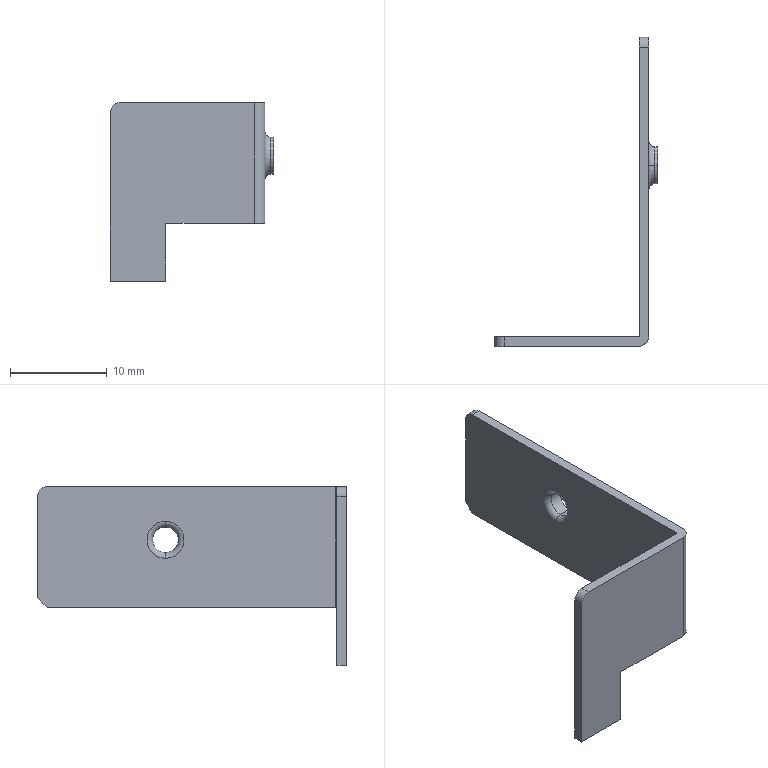Part | STEP file | LRS-150-12_X2_5F00517375-151333 | 1 solid | 24 faces | box 16.9 x 32 x 18.5 mm | volume 618.141 mm3 | plane 12 | cylinder 8 | torus 4 | commonest cylinder face diameters 2 x2 2.65 x2 3.85 x2 0.2 x1 2.2 x1